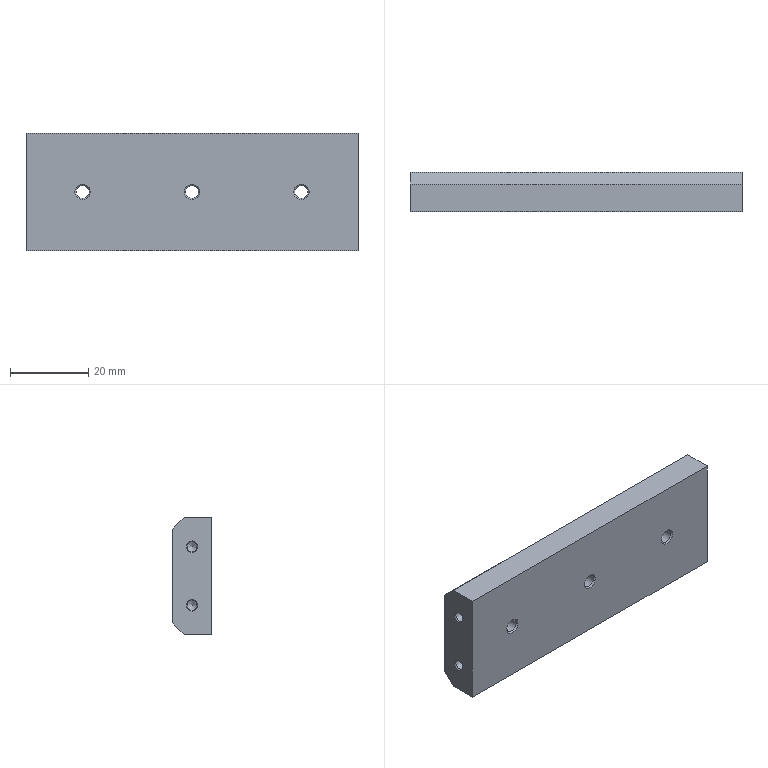Part | NX | features SIMPLE HOLE 7, SYMBOLIC_THREAD 7, DATUM_CSYS 5, SKETCH 4, HOLE PACKAGE 3, OFFSET_REGION 2, CHAMFER 1, EXTRUDE 1, LINKED_FACE 1 | 1 solid | 29 faces | box 85 x 10 x 30 mm | volume 24243 mm3 | cone 14 | plane 8 | cylinder 7 | commonest cylinder face diameters 2.5 x4 3.3 x3
STEP:
#1=CARTESIAN_POINT('',(-553.986,1030.061,354.782));
#2=VERTEX_POINT('',#1);
#3=CARTESIAN_POINT('',(-553.986,1030.061,356.782));
#4=DIRECTION('',(0.,-1.,0.));
#5=DIRECTION('',(0.,0.,-1.));
#6=AXIS2_PLACEMENT_3D('',#3,#4,#5);
#7=CIRCLE('',#6,2.);
#8=EDGE_CURVE('',#2,#2,#7,.T.);
#9=ORIENTED_EDGE('',*,*,#8,.T.);
#10=EDGE_LOOP('',(#9));
#11=FACE_BOUND('',#10,.T.);
#12=CARTESIAN_POINT('',(-581.986,1030.061,354.782));
#13=VERTEX_POINT('',#12);
#14=CARTESIAN_POINT('',(-581.986,1030.061,356.782));
#15=DIRECTION('',(0.,-1.,0.));
#16=DIRECTION('',(0.,0.,-1.));
#17=AXIS2_PLACEMENT_3D('',#14,#15,#16);
#18=CIRCLE('',#17,2.);
#19=EDGE_CURVE('',#13,#13,#18,.T.);
#20=ORIENTED_EDGE('',*,*,#19,.T.);
#21=EDGE_LOOP('',(#20));
#22=FACE_BOUND('',#21,.T.);
#23=CARTESIAN_POINT('',(-609.986,1030.061,354.782));
#24=VERTEX_POINT('',#23);
#25=CARTESIAN_POINT('',(-609.986,1030.061,356.782));
#26=DIRECTION('',(0.,-1.,0.));
#27=DIRECTION('',(0.,0.,-1.));
#28=AXIS2_PLACEMENT_3D('',#25,#26,#27);
#29=CIRCLE('',#28,2.);
#30=EDGE_CURVE('',#24,#24,#29,.T.);
#31=ORIENTED_EDGE('',*,*,#30,.T.);
#32=EDGE_LOOP('',(#31));
#33=FACE_BOUND('',#32,.T.);
#34=CARTESIAN_POINT('',(-539.486,1030.061,368.782));
#35=VERTEX_POINT('',#34);
#36=CARTESIAN_POINT('',(-539.486,1030.061,344.782));
#37=VERTEX_POINT('',#36);
#38=CARTESIAN_POINT('',(-539.486,1030.061,371.782));
#39=DIRECTION('',(0.,0.,-1.));
#40=VECTOR('',#39,1000.);
#41=LINE('',#38,#40);
#42=EDGE_CURVE('',#35,#37,#41,.T.);
#43=ORIENTED_EDGE('',*,*,#42,.T.);
#44=CARTESIAN_POINT('',(-624.486,1030.061,344.782));
#45=VERTEX_POINT('',#44);
#46=CARTESIAN_POINT('',(-538.986,1030.061,344.782));
#47=DIRECTION('',(-1.,0.,0.));
#48=VECTOR('',#47,1000.);
#49=LINE('',#46,#48);
#50=EDGE_CURVE('',#37,#45,#49,.T.);
#51=ORIENTED_EDGE('',*,*,#50,.T.);
#52=CARTESIAN_POINT('',(-624.486,1030.061,368.782));
#53=VERTEX_POINT('',#52);
#54=CARTESIAN_POINT('',(-624.486,1030.061,371.782));
#55=DIRECTION('',(0.,0.,-1.));
#56=VECTOR('',#55,1000.);
#57=LINE('',#54,#56);
#58=EDGE_CURVE('',#53,#45,#57,.T.);
#59=ORIENTED_EDGE('',*,*,#58,.F.);
#60=CARTESIAN_POINT('',(-538.986,1030.061,368.782));
#61=DIRECTION('',(1.,0.,0.));
#62=VECTOR('',#61,1000.);
#63=LINE('',#60,#62);
#64=EDGE_CURVE('',#53,#35,#63,.T.);
#65=ORIENTED_EDGE('',*,*,#64,.T.);
#66=EDGE_LOOP('',(#43,#51,#59,#65));
#67=FACE_BOUND('',#66,.T.);
#68=CARTESIAN_POINT('',(-538.986,1030.061,371.782));
#69=DIRECTION('',(0.,-1.,0.));
#70=DIRECTION('',(0.,0.,-1.));
#71=AXIS2_PLACEMENT_3D('',#68,#69,#70);
#72=PLANE('',#71);
#73=ADVANCED_FACE('',(#11,#22,#33,#67),#72,.F.);
#74=CARTESIAN_POINT('',(-624.486,1025.061,362.782));
#75=VERTEX_POINT('',#74);
#76=CARTESIAN_POINT('',(-624.486,1025.061,364.282));
#77=DIRECTION('',(1.,0.,0.));
#78=DIRECTION('',(0.,0.,-1.));
#79=AXIS2_PLACEMENT_3D('',#76,#77,#78);
#80=CIRCLE('',#79,1.5);
#81=EDGE_CURVE('',#75,#75,#80,.T.);
#82=ORIENTED_EDGE('',*,*,#81,.T.);
#83=EDGE_LOOP('',(#82));
#84=FACE_BOUND('',#83,.T.);
#85=CARTESIAN_POINT('',(-624.486,1025.061,347.782));
#86=VERTEX_POINT('',#85);
#87=CARTESIAN_POINT('',(-624.486,1025.061,349.282));
#88=DIRECTION('',(1.,0.,0.));
#89=DIRECTION('',(0.,0.,-1.));
#90=AXIS2_PLACEMENT_3D('',#87,#88,#89);
#91=CIRCLE('',#90,1.5);
#92=EDGE_CURVE('',#86,#86,#91,.T.);
#93=ORIENTED_EDGE('',*,*,#92,.T.);
#94=EDGE_LOOP('',(#93));
#95=FACE_BOUND('',#94,.T.);
#96=ORIENTED_EDGE('',*,*,#58,.T.);
#97=CARTESIAN_POINT('',(-624.486,1027.061,341.782));
#98=VERTEX_POINT('',#97);
#99=CARTESIAN_POINT('',(-624.486,1030.061,344.782));
#100=DIRECTION('',(0.,0.7071,0.7071));
#101=VECTOR('',#100,1000.);
#102=LINE('',#99,#101);
#103=EDGE_CURVE('',#45,#98,#102,.F.);
#104=ORIENTED_EDGE('',*,*,#103,.T.);
#105=CARTESIAN_POINT('',(-624.486,1020.061,341.782));
#106=VERTEX_POINT('',#105);
#107=CARTESIAN_POINT('',(-624.486,1030.061,341.782));
#108=DIRECTION('',(0.,-1.,0.));
#109=VECTOR('',#108,1000.);
#110=LINE('',#107,#109);
#111=EDGE_CURVE('',#98,#106,#110,.T.);
#112=ORIENTED_EDGE('',*,*,#111,.T.);
#113=CARTESIAN_POINT('',(-624.486,1020.061,371.782));
#114=VERTEX_POINT('',#113);
#115=CARTESIAN_POINT('',(-624.486,1020.061,371.782));
#116=DIRECTION('',(0.,0.,-1.));
#117=VECTOR('',#116,1000.);
#118=LINE('',#115,#117);
#119=EDGE_CURVE('',#114,#106,#118,.T.);
#120=ORIENTED_EDGE('',*,*,#119,.F.);
#121=CARTESIAN_POINT('',(-624.486,1027.061,371.782));
#122=VERTEX_POINT('',#121);
#123=CARTESIAN_POINT('',(-624.486,1030.061,371.782));
#124=DIRECTION('',(0.,-1.,0.));
#125=VECTOR('',#124,1000.);
#126=LINE('',#123,#125);
#127=EDGE_CURVE('',#122,#114,#126,.T.);
#128=ORIENTED_EDGE('',*,*,#127,.F.);
#129=CARTESIAN_POINT('',(-624.486,1027.061,371.782));
#130=DIRECTION('',(0.,0.7071,-0.7071));
#131=VECTOR('',#130,1000.);
#132=LINE('',#129,#131);
#133=EDGE_CURVE('',#122,#53,#132,.T.);
#134=ORIENTED_EDGE('',*,*,#133,.T.);
#135=EDGE_LOOP('',(#96,#104,#112,#120,#128,#134));
#136=FACE_BOUND('',#135,.T.);
#137=CARTESIAN_POINT('',(-624.486,1030.061,371.782));
#138=DIRECTION('',(1.,0.,0.));
#139=DIRECTION('',(0.,0.,-1.));
#140=AXIS2_PLACEMENT_3D('',#137,#138,#139);
#141=PLANE('',#140);
#142=ADVANCED_FACE('',(#84,#95,#136),#141,.F.);
#143=CARTESIAN_POINT('',(-553.986,1020.061,358.782));
#144=VERTEX_POINT('',#143);
#145=CARTESIAN_POINT('',(-553.986,1020.061,356.782));
#146=DIRECTION('',(0.,1.,0.));
#147=DIRECTION('',(0.,0.,1.));
#148=AXIS2_PLACEMENT_3D('',#145,#146,#147);
#149=CIRCLE('',#148,2.);
#150=EDGE_CURVE('',#144,#144,#149,.T.);
#151=ORIENTED_EDGE('',*,*,#150,.T.);
#152=EDGE_LOOP('',(#151));
#153=FACE_BOUND('',#152,.T.);
#154=CARTESIAN_POINT('',(-581.986,1020.061,358.782));
#155=VERTEX_POINT('',#154);
#156=CARTESIAN_POINT('',(-581.986,1020.061,356.782));
#157=DIRECTION('',(0.,1.,0.));
#158=DIRECTION('',(0.,0.,1.));
#159=AXIS2_PLACEMENT_3D('',#156,#157,#158);
#160=CIRCLE('',#159,2.);
#161=EDGE_CURVE('',#155,#155,#160,.T.);
#162=ORIENTED_EDGE('',*,*,#161,.T.);
#163=EDGE_LOOP('',(#162));
#164=FACE_BOUND('',#163,.T.);
#165=CARTESIAN_POINT('',(-609.986,1020.061,358.782));
#166=VERTEX_POINT('',#165);
#167=CARTESIAN_POINT('',(-609.986,1020.061,356.782));
#168=DIRECTION('',(0.,1.,0.));
#169=DIRECTION('',(0.,0.,1.));
#170=AXIS2_PLACEMENT_3D('',#167,#168,#169);
#171=CIRCLE('',#170,2.);
#172=EDGE_CURVE('',#166,#166,#171,.T.);
#173=ORIENTED_EDGE('',*,*,#172,.T.);
#174=EDGE_LOOP('',(#173));
#175=FACE_BOUND('',#174,.T.);
#176=CARTESIAN_POINT('',(-539.486,1020.061,341.782));
#177=VERTEX_POINT('',#176);
#178=CARTESIAN_POINT('',(-624.986,1020.061,341.782));
#179=DIRECTION('',(1.,0.,0.));
#180=VECTOR('',#179,1000.);
#181=LINE('',#178,#180);
#182=EDGE_CURVE('',#106,#177,#181,.T.);
#183=ORIENTED_EDGE('',*,*,#182,.T.);
#184=CARTESIAN_POINT('',(-539.486,1020.061,371.782));
#185=VERTEX_POINT('',#184);
#186=CARTESIAN_POINT('',(-539.486,1020.061,371.782));
#187=DIRECTION('',(0.,0.,-1.));
#188=VECTOR('',#187,1000.);
#189=LINE('',#186,#188);
#190=EDGE_CURVE('',#185,#177,#189,.T.);
#191=ORIENTED_EDGE('',*,*,#190,.F.);
#192=CARTESIAN_POINT('',(-624.986,1020.061,371.782));
#193=DIRECTION('',(1.,0.,0.));
#194=VECTOR('',#193,1000.);
#195=LINE('',#192,#194);
#196=EDGE_CURVE('',#114,#185,#195,.T.);
#197=ORIENTED_EDGE('',*,*,#196,.F.);
#198=ORIENTED_EDGE('',*,*,#119,.T.);
#199=EDGE_LOOP('',(#183,#191,#197,#198));
#200=FACE_BOUND('',#199,.T.);
#201=CARTESIAN_POINT('',(-624.986,1020.061,371.782));
#202=DIRECTION('',(0.,1.,0.));
#203=DIRECTION('',(0.,0.,1.));
#204=AXIS2_PLACEMENT_3D('',#201,#202,#203);
#205=PLANE('',#204);
#206=ADVANCED_FACE('',(#153,#164,#175,#200),#205,.F.);
#207=CARTESIAN_POINT('',(-539.486,1025.061,365.782));
#208=VERTEX_POINT('',#207);
#209=CARTESIAN_POINT('',(-539.486,1025.061,364.282));
#210=DIRECTION('',(-1.,0.,0.));
#211=DIRECTION('',(0.,0.,1.));
#212=AXIS2_PLACEMENT_3D('',#209,#210,#211);
#213=CIRCLE('',#212,1.5);
#214=EDGE_CURVE('',#208,#208,#213,.T.);
#215=ORIENTED_EDGE('',*,*,#214,.T.);
#216=EDGE_LOOP('',(#215));
#217=FACE_BOUND('',#216,.T.);
#218=CARTESIAN_POINT('',(-539.486,1025.061,350.782));
#219=VERTEX_POINT('',#218);
#220=CARTESIAN_POINT('',(-539.486,1025.061,349.282));
#221=DIRECTION('',(-1.,0.,0.));
#222=DIRECTION('',(0.,0.,1.));
#223=AXIS2_PLACEMENT_3D('',#220,#221,#222);
#224=CIRCLE('',#223,1.5);
#225=EDGE_CURVE('',#219,#219,#224,.T.);
#226=ORIENTED_EDGE('',*,*,#225,.T.);
#227=EDGE_LOOP('',(#226));
#228=FACE_BOUND('',#227,.T.);
#229=CARTESIAN_POINT('',(-539.486,1027.061,341.782));
#230=VERTEX_POINT('',#229);
#231=CARTESIAN_POINT('',(-539.486,1020.061,341.782));
#232=DIRECTION('',(0.,1.,0.));
#233=VECTOR('',#232,1000.);
#234=LINE('',#231,#233);
#235=EDGE_CURVE('',#177,#230,#234,.T.);
#236=ORIENTED_EDGE('',*,*,#235,.T.);
#237=CARTESIAN_POINT('',(-539.486,1030.061,344.782));
#238=DIRECTION('',(0.,-0.7071,-0.7071));
#239=VECTOR('',#238,1000.);
#240=LINE('',#237,#239);
#241=EDGE_CURVE('',#230,#37,#240,.F.);
#242=ORIENTED_EDGE('',*,*,#241,.T.);
#243=ORIENTED_EDGE('',*,*,#42,.F.);
#244=CARTESIAN_POINT('',(-539.486,1027.061,371.782));
#245=VERTEX_POINT('',#244);
#246=CARTESIAN_POINT('',(-539.486,1027.061,371.782));
#247=DIRECTION('',(0.,-0.7071,0.7071));
#248=VECTOR('',#247,1000.);
#249=LINE('',#246,#248);
#250=EDGE_CURVE('',#35,#245,#249,.T.);
#251=ORIENTED_EDGE('',*,*,#250,.T.);
#252=CARTESIAN_POINT('',(-539.486,1020.061,371.782));
#253=DIRECTION('',(0.,1.,0.));
#254=VECTOR('',#253,1000.);
#255=LINE('',#252,#254);
#256=EDGE_CURVE('',#185,#245,#255,.T.);
#257=ORIENTED_EDGE('',*,*,#256,.F.);
#258=ORIENTED_EDGE('',*,*,#190,.T.);
#259=EDGE_LOOP('',(#236,#242,#243,#251,#257,#258));
#260=FACE_BOUND('',#259,.T.);
#261=CARTESIAN_POINT('',(-539.486,1020.061,371.782));
#262=DIRECTION('',(-1.,0.,0.));
#263=DIRECTION('',(0.,0.,1.));
#264=AXIS2_PLACEMENT_3D('',#261,#262,#263);
#265=PLANE('',#264);
#266=ADVANCED_FACE('',(#217,#228,#260),#265,.F.);
#267=ORIENTED_EDGE('',*,*,#256,.T.);
#268=CARTESIAN_POINT('',(-624.986,1027.061,371.782));
#269=DIRECTION('',(-1.,0.,0.));
#270=VECTOR('',#269,1000.);
#271=LINE('',#268,#270);
#272=EDGE_CURVE('',#245,#122,#271,.T.);
#273=ORIENTED_EDGE('',*,*,#272,.T.);
#274=ORIENTED_EDGE('',*,*,#127,.T.);
#275=ORIENTED_EDGE('',*,*,#196,.T.);
#276=EDGE_LOOP('',(#267,#273,#274,#275));
#277=FACE_BOUND('',#276,.T.);
#278=CARTESIAN_POINT('',(0.,0.,371.782));
#279=DIRECTION('',(0.,0.,1.));
#280=DIRECTION('',(1.,0.,0.));
#281=AXIS2_PLACEMENT_3D('',#278,#279,#280);
#282=PLANE('',#281);
#283=ADVANCED_FACE('',(#277),#282,.T.);
#284=ORIENTED_EDGE('',*,*,#111,.F.);
#285=CARTESIAN_POINT('',(0.,1027.061,341.782));
#286=DIRECTION('',(1.,0.,0.));
#287=VECTOR('',#286,1000.);
#288=LINE('',#285,#287);
#289=EDGE_CURVE('',#98,#230,#288,.T.);
#290=ORIENTED_EDGE('',*,*,#289,.T.);
#291=ORIENTED_EDGE('',*,*,#235,.F.);
#292=ORIENTED_EDGE('',*,*,#182,.F.);
#293=EDGE_LOOP('',(#284,#290,#291,#292));
#294=FACE_BOUND('',#293,.T.);
#295=CARTESIAN_POINT('',(0.,0.,341.782));
#296=DIRECTION('',(0.,0.,1.));
#297=DIRECTION('',(1.,0.,0.));
#298=AXIS2_PLACEMENT_3D('',#295,#296,#297);
#299=PLANE('',#298);
#300=ADVANCED_FACE('',(#294),#299,.F.);
#301=ORIENTED_EDGE('',*,*,#241,.F.);
#302=ORIENTED_EDGE('',*,*,#289,.F.);
#303=ORIENTED_EDGE('',*,*,#103,.F.);
#304=ORIENTED_EDGE('',*,*,#50,.F.);
#305=EDGE_LOOP('',(#301,#302,#303,#304));
#306=FACE_BOUND('',#305,.T.);
#307=CARTESIAN_POINT('',(-538.986,1030.061,344.782));
#308=DIRECTION('',(0.,-0.7071,0.7071));
#309=DIRECTION('',(-1.,0.,0.));
#310=AXIS2_PLACEMENT_3D('',#307,#308,#309);
#311=PLANE('',#310);
#312=ADVANCED_FACE('',(#306),#311,.F.);
#313=ORIENTED_EDGE('',*,*,#250,.F.);
#314=ORIENTED_EDGE('',*,*,#64,.F.);
#315=ORIENTED_EDGE('',*,*,#133,.F.);
#316=ORIENTED_EDGE('',*,*,#272,.F.);
#317=EDGE_LOOP('',(#313,#314,#315,#316));
#318=FACE_BOUND('',#317,.T.);
#319=CARTESIAN_POINT('',(0.,1027.061,371.782));
#320=DIRECTION('',(0.,0.7071,0.7071));
#321=DIRECTION('',(1.,0.,0.));
#322=AXIS2_PLACEMENT_3D('',#319,#320,#321);
#323=PLANE('',#322);
#324=ADVANCED_FACE('',(#318),#323,.T.);
#325=CARTESIAN_POINT('',(-609.986,1029.711,355.132));
#326=VERTEX_POINT('',#325);
#327=CARTESIAN_POINT('',(-609.986,1029.711,356.782));
#328=DIRECTION('',(0.,-1.,0.));
#329=DIRECTION('',(0.,0.,-1.));
#330=AXIS2_PLACEMENT_3D('',#327,#328,#329);
#331=CIRCLE('',#330,1.65);
#332=EDGE_CURVE('',#326,#326,#331,.F.);
#333=ORIENTED_EDGE('',*,*,#332,.T.);
#334=EDGE_LOOP('',(#333));
#335=FACE_BOUND('',#334,.T.);
#336=CARTESIAN_POINT('',(-609.986,1020.411,358.432));
#337=VERTEX_POINT('',#336);
#338=CARTESIAN_POINT('',(-609.986,1020.411,356.782));
#339=DIRECTION('',(0.,1.,0.));
#340=DIRECTION('',(0.,0.,1.));
#341=AXIS2_PLACEMENT_3D('',#338,#339,#340);
#342=CIRCLE('',#341,1.65);
#343=EDGE_CURVE('',#337,#337,#342,.F.);
#344=ORIENTED_EDGE('',*,*,#343,.T.);
#345=EDGE_LOOP('',(#344));
#346=FACE_BOUND('',#345,.T.);
#347=CARTESIAN_POINT('',(-609.986,1020.061,356.782));
#348=DIRECTION('',(0.,1.,0.));
#349=DIRECTION('',(0.,0.,1.));
#350=AXIS2_PLACEMENT_3D('',#347,#348,#349);
#351=CYLINDRICAL_SURFACE('',#350,1.65);
#352=ADVANCED_FACE('',(#335,#346),#351,.F.);
#353=ORIENTED_EDGE('',*,*,#343,.F.);
#354=EDGE_LOOP('',(#353));
#355=FACE_BOUND('',#354,.T.);
#356=ORIENTED_EDGE('',*,*,#172,.F.);
#357=EDGE_LOOP('',(#356));
#358=FACE_BOUND('',#357,.T.);
#359=CARTESIAN_POINT('',(-609.986,1020.061,356.782));
#360=DIRECTION('',(0.,-1.,0.));
#361=DIRECTION('',(0.,0.,-1.));
#362=AXIS2_PLACEMENT_3D('',#359,#360,#361);
#363=CONICAL_SURFACE('',#362,2.,0.7854);
#364=ADVANCED_FACE('',(#355,#358),#363,.F.);
#365=ORIENTED_EDGE('',*,*,#332,.F.);
#366=EDGE_LOOP('',(#365));
#367=FACE_BOUND('',#366,.T.);
#368=ORIENTED_EDGE('',*,*,#30,.F.);
#369=EDGE_LOOP('',(#368));
#370=FACE_BOUND('',#369,.T.);
#371=CARTESIAN_POINT('',(-609.986,1030.061,356.782));
#372=DIRECTION('',(0.,1.,0.));
#373=DIRECTION('',(0.,0.,1.));
#374=AXIS2_PLACEMENT_3D('',#371,#372,#373);
#375=CONICAL_SURFACE('',#374,2.,0.7854);
#376=ADVANCED_FACE('',(#367,#370),#375,.F.);
#377=CARTESIAN_POINT('',(-581.986,1029.711,355.132));
#378=VERTEX_POINT('',#377);
#379=CARTESIAN_POINT('',(-581.986,1029.711,356.782));
#380=DIRECTION('',(0.,-1.,0.));
#381=DIRECTION('',(0.,0.,-1.));
#382=AXIS2_PLACEMENT_3D('',#379,#380,#381);
#383=CIRCLE('',#382,1.65);
#384=EDGE_CURVE('',#378,#378,#383,.F.);
#385=ORIENTED_EDGE('',*,*,#384,.T.);
#386=EDGE_LOOP('',(#385));
#387=FACE_BOUND('',#386,.T.);
#388=CARTESIAN_POINT('',(-581.986,1020.411,358.432));
#389=VERTEX_POINT('',#388);
#390=CARTESIAN_POINT('',(-581.986,1020.411,356.782));
#391=DIRECTION('',(0.,1.,0.));
#392=DIRECTION('',(0.,0.,1.));
#393=AXIS2_PLACEMENT_3D('',#390,#391,#392);
#394=CIRCLE('',#393,1.65);
#395=EDGE_CURVE('',#389,#389,#394,.F.);
#396=ORIENTED_EDGE('',*,*,#395,.T.);
#397=EDGE_LOOP('',(#396));
#398=FACE_BOUND('',#397,.T.);
#399=CARTESIAN_POINT('',(-581.986,1020.061,356.782));
#400=DIRECTION('',(0.,1.,0.));
#401=DIRECTION('',(0.,0.,1.));
#402=AXIS2_PLACEMENT_3D('',#399,#400,#401);
#403=CYLINDRICAL_SURFACE('',#402,1.65);
#404=ADVANCED_FACE('',(#387,#398),#403,.F.);
#405=ORIENTED_EDGE('',*,*,#395,.F.);
#406=EDGE_LOOP('',(#405));
#407=FACE_BOUND('',#406,.T.);
#408=ORIENTED_EDGE('',*,*,#161,.F.);
#409=EDGE_LOOP('',(#408));
#410=FACE_BOUND('',#409,.T.);
#411=CARTESIAN_POINT('',(-581.986,1020.061,356.782));
#412=DIRECTION('',(0.,-1.,0.));
#413=DIRECTION('',(0.,0.,-1.));
#414=AXIS2_PLACEMENT_3D('',#411,#412,#413);
#415=CONICAL_SURFACE('',#414,2.,0.7854);
#416=ADVANCED_FACE('',(#407,#410),#415,.F.);
#417=ORIENTED_EDGE('',*,*,#384,.F.);
#418=EDGE_LOOP('',(#417));
#419=FACE_BOUND('',#418,.T.);
#420=ORIENTED_EDGE('',*,*,#19,.F.);
#421=EDGE_LOOP('',(#420));
#422=FACE_BOUND('',#421,.T.);
#423=CARTESIAN_POINT('',(-581.986,1030.061,356.782));
#424=DIRECTION('',(0.,1.,0.));
#425=DIRECTION('',(0.,0.,1.));
#426=AXIS2_PLACEMENT_3D('',#423,#424,#425);
#427=CONICAL_SURFACE('',#426,2.,0.7854);
#428=ADVANCED_FACE('',(#419,#422),#427,.F.);
#429=CARTESIAN_POINT('',(-553.986,1029.711,355.132));
#430=VERTEX_POINT('',#429);
#431=CARTESIAN_POINT('',(-553.986,1029.711,356.782));
#432=DIRECTION('',(0.,-1.,0.));
#433=DIRECTION('',(0.,0.,-1.));
#434=AXIS2_PLACEMENT_3D('',#431,#432,#433);
#435=CIRCLE('',#434,1.65);
#436=EDGE_CURVE('',#430,#430,#435,.F.);
#437=ORIENTED_EDGE('',*,*,#436,.T.);
#438=EDGE_LOOP('',(#437));
#439=FACE_BOUND('',#438,.T.);
#440=CARTESIAN_POINT('',(-553.986,1020.411,358.432));
#441=VERTEX_POINT('',#440);
#442=CARTESIAN_POINT('',(-553.986,1020.411,356.782));
#443=DIRECTION('',(0.,1.,0.));
#444=DIRECTION('',(0.,0.,1.));
#445=AXIS2_PLACEMENT_3D('',#442,#443,#444);
#446=CIRCLE('',#445,1.65);
#447=EDGE_CURVE('',#441,#441,#446,.F.);
#448=ORIENTED_EDGE('',*,*,#447,.T.);
#449=EDGE_LOOP('',(#448));
#450=FACE_BOUND('',#449,.T.);
#451=CARTESIAN_POINT('',(-553.986,1020.061,356.782));
#452=DIRECTION('',(0.,1.,0.));
#453=DIRECTION('',(0.,0.,1.));
#454=AXIS2_PLACEMENT_3D('',#451,#452,#453);
#455=CYLINDRICAL_SURFACE('',#454,1.65);
#456=ADVANCED_FACE('',(#439,#450),#455,.F.);
#457=ORIENTED_EDGE('',*,*,#447,.F.);
#458=EDGE_LOOP('',(#457));
#459=FACE_BOUND('',#458,.T.);
#460=ORIENTED_EDGE('',*,*,#150,.F.);
#461=EDGE_LOOP('',(#460));
#462=FACE_BOUND('',#461,.T.);
#463=CARTESIAN_POINT('',(-553.986,1020.061,356.782));
#464=DIRECTION('',(0.,-1.,0.));
#465=DIRECTION('',(0.,0.,-1.));
#466=AXIS2_PLACEMENT_3D('',#463,#464,#465);
#467=CONICAL_SURFACE('',#466,2.,0.7854);
#468=ADVANCED_FACE('',(#459,#462),#467,.F.);
#469=ORIENTED_EDGE('',*,*,#436,.F.);
#470=EDGE_LOOP('',(#469));
#471=FACE_BOUND('',#470,.T.);
#472=ORIENTED_EDGE('',*,*,#8,.F.);
#473=EDGE_LOOP('',(#472));
#474=FACE_BOUND('',#473,.T.);
#475=CARTESIAN_POINT('',(-553.986,1030.061,356.782));
#476=DIRECTION('',(0.,1.,0.));
#477=DIRECTION('',(0.,0.,1.));
#478=AXIS2_PLACEMENT_3D('',#475,#476,#477);
#479=CONICAL_SURFACE('',#478,2.,0.7854);
#480=ADVANCED_FACE('',(#471,#474),#479,.F.);
#481=CARTESIAN_POINT('',(-550.986,1025.061,350.532));
#482=VERTEX_POINT('',#481);
#483=CARTESIAN_POINT('',(-550.986,1025.061,349.282));
#484=DIRECTION('',(-1.,0.,0.));
#485=DIRECTION('',(0.,0.,1.));
#486=AXIS2_PLACEMENT_3D('',#483,#484,#485);
#487=CIRCLE('',#486,1.25);
#488=EDGE_CURVE('',#482,#482,#487,.F.);
#489=ORIENTED_EDGE('',*,*,#488,.T.);
#490=EDGE_LOOP('',(#489));
#491=FACE_BOUND('',#490,.T.);
#492=CARTESIAN_POINT('',(-551.737,1025.061,349.282));
#493=VERTEX_POINT('',#492);
#494=VERTEX_LOOP('',#493);
#495=FACE_BOUND('',#494,.T.);
#496=CARTESIAN_POINT('',(-550.986,1025.061,349.282));
#497=DIRECTION('',(1.,0.,0.));
#498=DIRECTION('',(0.,0.,-1.));
#499=AXIS2_PLACEMENT_3D('',#496,#497,#498);
#500=CONICAL_SURFACE('',#499,1.25,1.03);
#501=ADVANCED_FACE('',(#491,#495),#500,.F.);
#502=CARTESIAN_POINT('',(-539.736,1025.061,348.032));
#503=VERTEX_POINT('',#502);
#504=CARTESIAN_POINT('',(-539.736,1025.061,349.282));
#505=DIRECTION('',(1.,0.,0.));
#506=DIRECTION('',(0.,0.,-1.));
#507=AXIS2_PLACEMENT_3D('',#504,#505,#506);
#508=CIRCLE('',#507,1.25);
#509=EDGE_CURVE('',#503,#503,#508,.T.);
#510=ORIENTED_EDGE('',*,*,#509,.T.);
#511=EDGE_LOOP('',(#510));
#512=FACE_BOUND('',#511,.T.);
#513=ORIENTED_EDGE('',*,*,#488,.F.);
#514=EDGE_LOOP('',(#513));
#515=FACE_BOUND('',#514,.T.);
#516=CARTESIAN_POINT('',(-538.986,1025.061,349.282));
#517=DIRECTION('',(-1.,0.,0.));
#518=DIRECTION('',(0.,0.,1.));
#519=AXIS2_PLACEMENT_3D('',#516,#517,#518);
#520=CYLINDRICAL_SURFACE('',#519,1.25);
#521=ADVANCED_FACE('',(#512,#515),#520,.F.);
#522=ORIENTED_EDGE('',*,*,#509,.F.);
#523=EDGE_LOOP('',(#522));
#524=FACE_BOUND('',#523,.T.);
#525=ORIENTED_EDGE('',*,*,#225,.F.);
#526=EDGE_LOOP('',(#525));
#527=FACE_BOUND('',#526,.T.);
#528=CARTESIAN_POINT('',(-539.486,1025.061,349.282));
#529=DIRECTION('',(1.,0.,0.));
#530=DIRECTION('',(0.,0.,-1.));
#531=AXIS2_PLACEMENT_3D('',#528,#529,#530);
#532=CONICAL_SURFACE('',#531,1.5,0.7854);
#533=ADVANCED_FACE('',(#524,#527),#532,.F.);
#534=CARTESIAN_POINT('',(-550.986,1025.061,365.532));
#535=VERTEX_POINT('',#534);
#536=CARTESIAN_POINT('',(-550.986,1025.061,364.282));
#537=DIRECTION('',(-1.,0.,0.));
#538=DIRECTION('',(0.,0.,1.));
#539=AXIS2_PLACEMENT_3D('',#536,#537,#538);
#540=CIRCLE('',#539,1.25);
#541=EDGE_CURVE('',#535,#535,#540,.F.);
#542=ORIENTED_EDGE('',*,*,#541,.T.);
#543=EDGE_LOOP('',(#542));
#544=FACE_BOUND('',#543,.T.);
#545=CARTESIAN_POINT('',(-551.737,1025.061,364.282));
#546=VERTEX_POINT('',#545);
#547=VERTEX_LOOP('',#546);
#548=FACE_BOUND('',#547,.T.);
#549=CARTESIAN_POINT('',(-550.986,1025.061,364.282));
#550=DIRECTION('',(1.,0.,0.));
#551=DIRECTION('',(0.,0.,-1.));
#552=AXIS2_PLACEMENT_3D('',#549,#550,#551);
#553=CONICAL_SURFACE('',#552,1.25,1.03);
#554=ADVANCED_FACE('',(#544,#548),#553,.F.);
#555=CARTESIAN_POINT('',(-539.736,1025.061,363.032));
#556=VERTEX_POINT('',#555);
#557=CARTESIAN_POINT('',(-539.736,1025.061,364.282));
#558=DIRECTION('',(1.,0.,0.));
#559=DIRECTION('',(0.,0.,-1.));
#560=AXIS2_PLACEMENT_3D('',#557,#558,#559);
#561=CIRCLE('',#560,1.25);
#562=EDGE_CURVE('',#556,#556,#561,.T.);
#563=ORIENTED_EDGE('',*,*,#562,.T.);
#564=EDGE_LOOP('',(#563));
#565=FACE_BOUND('',#564,.T.);
#566=ORIENTED_EDGE('',*,*,#541,.F.);
#567=EDGE_LOOP('',(#566));
#568=FACE_BOUND('',#567,.T.);
#569=CARTESIAN_POINT('',(-538.986,1025.061,364.282));
#570=DIRECTION('',(-1.,0.,0.));
#571=DIRECTION('',(0.,0.,1.));
#572=AXIS2_PLACEMENT_3D('',#569,#570,#571);
#573=CYLINDRICAL_SURFACE('',#572,1.25);
#574=ADVANCED_FACE('',(#565,#568),#573,.F.);
#575=ORIENTED_EDGE('',*,*,#562,.F.);
#576=EDGE_LOOP('',(#575));
#577=FACE_BOUND('',#576,.T.);
#578=ORIENTED_EDGE('',*,*,#214,.F.);
#579=EDGE_LOOP('',(#578));
#580=FACE_BOUND('',#579,.T.);
#581=CARTESIAN_POINT('',(-539.486,1025.061,364.282));
#582=DIRECTION('',(1.,0.,0.));
#583=DIRECTION('',(0.,0.,-1.));
#584=AXIS2_PLACEMENT_3D('',#581,#582,#583);
#585=CONICAL_SURFACE('',#584,1.5,0.7854);
#586=ADVANCED_FACE('',(#577,#580),#585,.F.);
#587=CARTESIAN_POINT('',(-612.986,1025.061,348.032));
#588=VERTEX_POINT('',#587);
#589=CARTESIAN_POINT('',(-612.986,1025.061,349.282));
#590=DIRECTION('',(1.,0.,0.));
#591=DIRECTION('',(0.,0.,-1.));
#592=AXIS2_PLACEMENT_3D('',#589,#590,#591);
#593=CIRCLE('',#592,1.25);
#594=EDGE_CURVE('',#588,#588,#593,.F.);
#595=ORIENTED_EDGE('',*,*,#594,.T.);
#596=EDGE_LOOP('',(#595));
#597=FACE_BOUND('',#596,.T.);
#598=CARTESIAN_POINT('',(-612.235,1025.061,349.282));
#599=VERTEX_POINT('',#598);
#600=VERTEX_LOOP('',#599);
#601=FACE_BOUND('',#600,.T.);
#602=CARTESIAN_POINT('',(-612.986,1025.061,349.282));
#603=DIRECTION('',(-1.,0.,0.));
#604=DIRECTION('',(0.,0.,1.));
#605=AXIS2_PLACEMENT_3D('',#602,#603,#604);
#606=CONICAL_SURFACE('',#605,1.25,1.03);
#607=ADVANCED_FACE('',(#597,#601),#606,.F.);
#608=CARTESIAN_POINT('',(-624.236,1025.061,350.532));
#609=VERTEX_POINT('',#608);
#610=CARTESIAN_POINT('',(-624.236,1025.061,349.282));
#611=DIRECTION('',(-1.,0.,0.));
#612=DIRECTION('',(0.,0.,1.));
#613=AXIS2_PLACEMENT_3D('',#610,#611,#612);
#614=CIRCLE('',#613,1.25);
#615=EDGE_CURVE('',#609,#609,#614,.T.);
#616=ORIENTED_EDGE('',*,*,#615,.T.);
#617=EDGE_LOOP('',(#616));
#618=FACE_BOUND('',#617,.T.);
#619=ORIENTED_EDGE('',*,*,#594,.F.);
#620=EDGE_LOOP('',(#619));
#621=FACE_BOUND('',#620,.T.);
#622=CARTESIAN_POINT('',(-624.986,1025.061,349.282));
#623=DIRECTION('',(1.,0.,0.));
#624=DIRECTION('',(0.,0.,-1.));
#625=AXIS2_PLACEMENT_3D('',#622,#623,#624);
#626=CYLINDRICAL_SURFACE('',#625,1.25);
#627=ADVANCED_FACE('',(#618,#621),#626,.F.);
#628=ORIENTED_EDGE('',*,*,#615,.F.);
#629=EDGE_LOOP('',(#628));
#630=FACE_BOUND('',#629,.T.);
#631=ORIENTED_EDGE('',*,*,#92,.F.);
#632=EDGE_LOOP('',(#631));
#633=FACE_BOUND('',#632,.T.);
#634=CARTESIAN_POINT('',(-624.486,1025.061,349.282));
#635=DIRECTION('',(-1.,0.,0.));
#636=DIRECTION('',(0.,0.,1.));
#637=AXIS2_PLACEMENT_3D('',#634,#635,#636);
#638=CONICAL_SURFACE('',#637,1.5,0.7854);
#639=ADVANCED_FACE('',(#630,#633),#638,.F.);
#640=CARTESIAN_POINT('',(-612.986,1025.061,363.032));
#641=VERTEX_POINT('',#640);
#642=CARTESIAN_POINT('',(-612.986,1025.061,364.282));
#643=DIRECTION('',(1.,0.,0.));
#644=DIRECTION('',(0.,0.,-1.));
#645=AXIS2_PLACEMENT_3D('',#642,#643,#644);
#646=CIRCLE('',#645,1.25);
#647=EDGE_CURVE('',#641,#641,#646,.F.);
#648=ORIENTED_EDGE('',*,*,#647,.T.);
#649=EDGE_LOOP('',(#648));
#650=FACE_BOUND('',#649,.T.);
#651=CARTESIAN_POINT('',(-612.235,1025.061,364.282));
#652=VERTEX_POINT('',#651);
#653=VERTEX_LOOP('',#652);
#654=FACE_BOUND('',#653,.T.);
#655=CARTESIAN_POINT('',(-612.986,1025.061,364.282));
#656=DIRECTION('',(-1.,0.,0.));
#657=DIRECTION('',(0.,0.,1.));
#658=AXIS2_PLACEMENT_3D('',#655,#656,#657);
#659=CONICAL_SURFACE('',#658,1.25,1.03);
#660=ADVANCED_FACE('',(#650,#654),#659,.F.);
#661=CARTESIAN_POINT('',(-624.236,1025.061,365.532));
#662=VERTEX_POINT('',#661);
#663=CARTESIAN_POINT('',(-624.236,1025.061,364.282));
#664=DIRECTION('',(-1.,0.,0.));
#665=DIRECTION('',(0.,0.,1.));
#666=AXIS2_PLACEMENT_3D('',#663,#664,#665);
#667=CIRCLE('',#666,1.25);
#668=EDGE_CURVE('',#662,#662,#667,.T.);
#669=ORIENTED_EDGE('',*,*,#668,.T.);
#670=EDGE_LOOP('',(#669));
#671=FACE_BOUND('',#670,.T.);
#672=ORIENTED_EDGE('',*,*,#647,.F.);
#673=EDGE_LOOP('',(#672));
#674=FACE_BOUND('',#673,.T.);
#675=CARTESIAN_POINT('',(-624.986,1025.061,364.282));
#676=DIRECTION('',(1.,0.,0.));
#677=DIRECTION('',(0.,0.,-1.));
#678=AXIS2_PLACEMENT_3D('',#675,#676,#677);
#679=CYLINDRICAL_SURFACE('',#678,1.25);
#680=ADVANCED_FACE('',(#671,#674),#679,.F.);
#681=ORIENTED_EDGE('',*,*,#668,.F.);
#682=EDGE_LOOP('',(#681));
#683=FACE_BOUND('',#682,.T.);
#684=ORIENTED_EDGE('',*,*,#81,.F.);
#685=EDGE_LOOP('',(#684));
#686=FACE_BOUND('',#685,.T.);
#687=CARTESIAN_POINT('',(-624.486,1025.061,364.282));
#688=DIRECTION('',(-1.,0.,0.));
#689=DIRECTION('',(0.,0.,1.));
#690=AXIS2_PLACEMENT_3D('',#687,#688,#689);
#691=CONICAL_SURFACE('',#690,1.5,0.7854);
#692=ADVANCED_FACE('',(#683,#686),#691,.F.);
#693=CLOSED_SHELL('',(#73,#142,#206,#266,#283,#300,#312,#324,#352,#364,#376,#404,#416,#428,#456,#468,#480,#501,#521,#533,#554,#574,#586,#607,#627,#639,#660,#680,#692));
#694=MANIFOLD_SOLID_BREP('',#693);
#695=(LENGTH_UNIT()NAMED_UNIT(*)SI_UNIT(.MILLI.,.METRE.));
#696=UNCERTAINTY_MEASURE_WITH_UNIT(LENGTH_MEASURE(0.00001),#695,'','');
#697=(NAMED_UNIT(*)PLANE_ANGLE_UNIT()SI_UNIT($,.RADIAN.));
#698=(NAMED_UNIT(*)SI_UNIT($,.STERADIAN.)SOLID_ANGLE_UNIT());
#699=(GEOMETRIC_REPRESENTATION_CONTEXT(3)GLOBAL_UNCERTAINTY_ASSIGNED_CONTEXT((#696))GLOBAL_UNIT_ASSIGNED_CONTEXT((#695,#697,#698))REPRESENTATION_CONTEXT('',''));
#700=ADVANCED_BREP_SHAPE_REPRESENTATION('',(#694),#699);